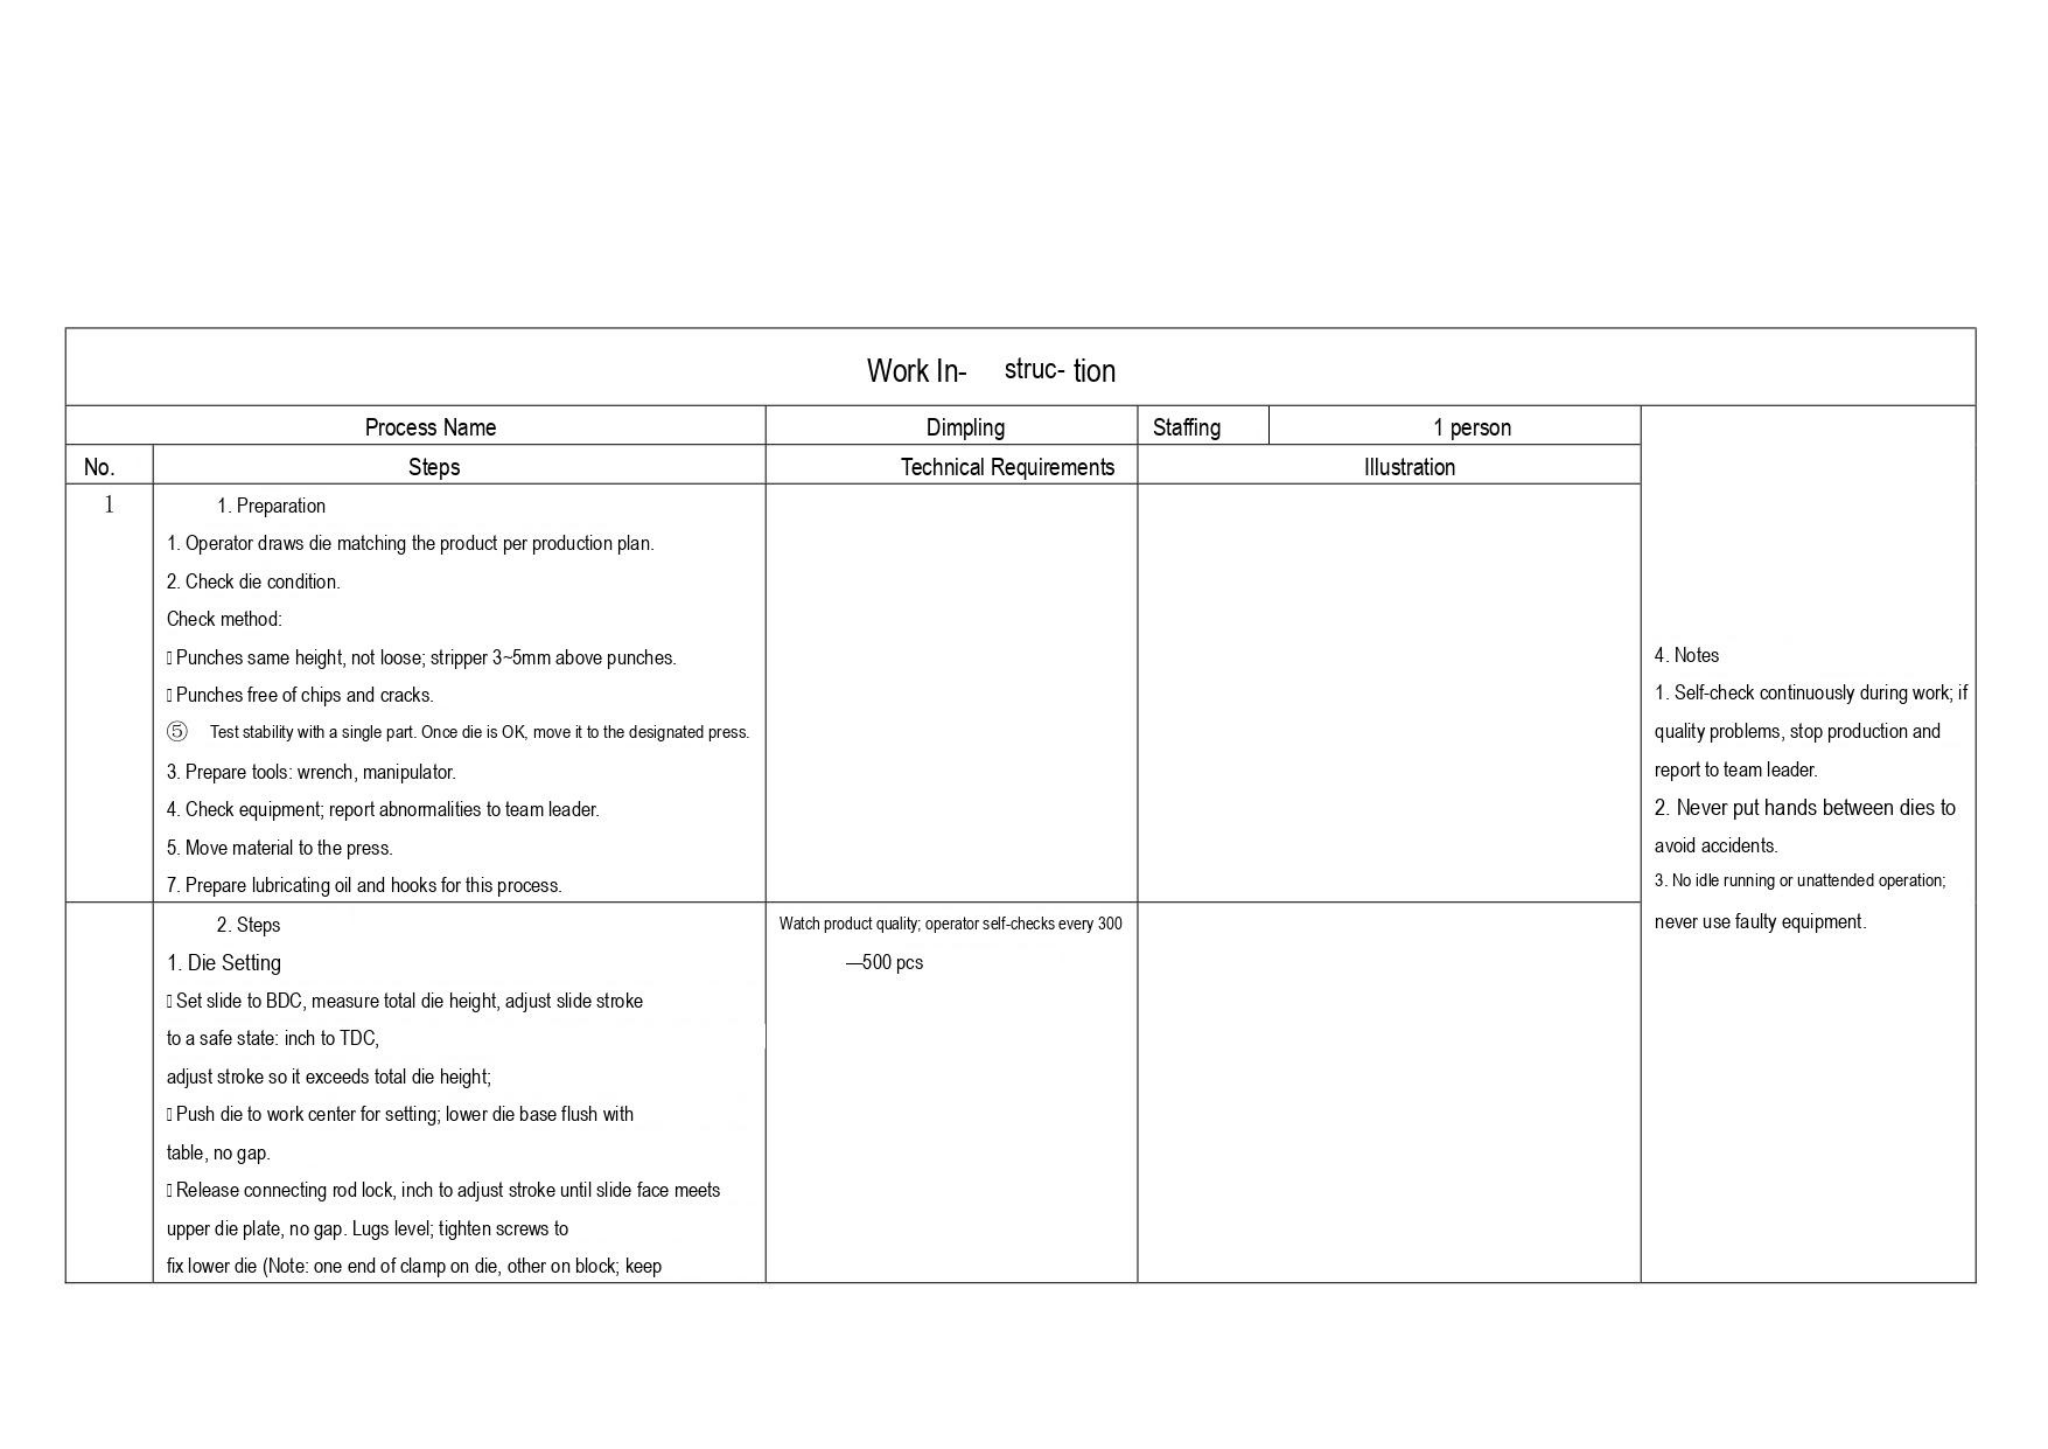# Work In- struc- tion

| Process Name | | Dimpling | Staffing | 1 person | |
|---|---|---|---|---|---|
| No. | Steps | Technical Requirements | Illustration | | |
| 1 | 1. Preparation<br>1. Operator draws die matching the product per production plan.<br>2. Check die condition.<br>Check method:<br>▯ Punches same height, not loose; stripper 3~5mm above punches.<br>▯ Punches free of chips and cracks.<br>⑤ Test stability with a single part. Once die is OK, move it to the designated press.<br>3. Prepare tools: wrench, manipulator.<br>4. Check equipment; report abnormalities to team leader.<br>5. Move material to the press.<br>7. Prepare lubricating oil and hooks for this process. | | | | 4. Notes<br>1. Self-check continuously during work; if quality problems, stop production and report to team leader.<br>2. Never put hands between dies to avoid accidents.<br>3. No idle running or unattended operation; never use faulty equipment. |
| | 2. Steps<br>1. Die Setting<br>▯ Set slide to BDC, measure total die height, adjust slide stroke to a safe state: inch to TDC,<br>adjust stroke so it exceeds total die height;<br>▯ Push die to work center for setting; lower die base flush with table, no gap.<br>▯ Release connecting rod lock, inch to adjust stroke until slide face meets upper die plate, no gap. Lugs level; tighten screws to fix lower die (Note: one end of clamp on die, other on block; keep | Watch product quality; operator self-checks every 300 —500 pcs | | | |
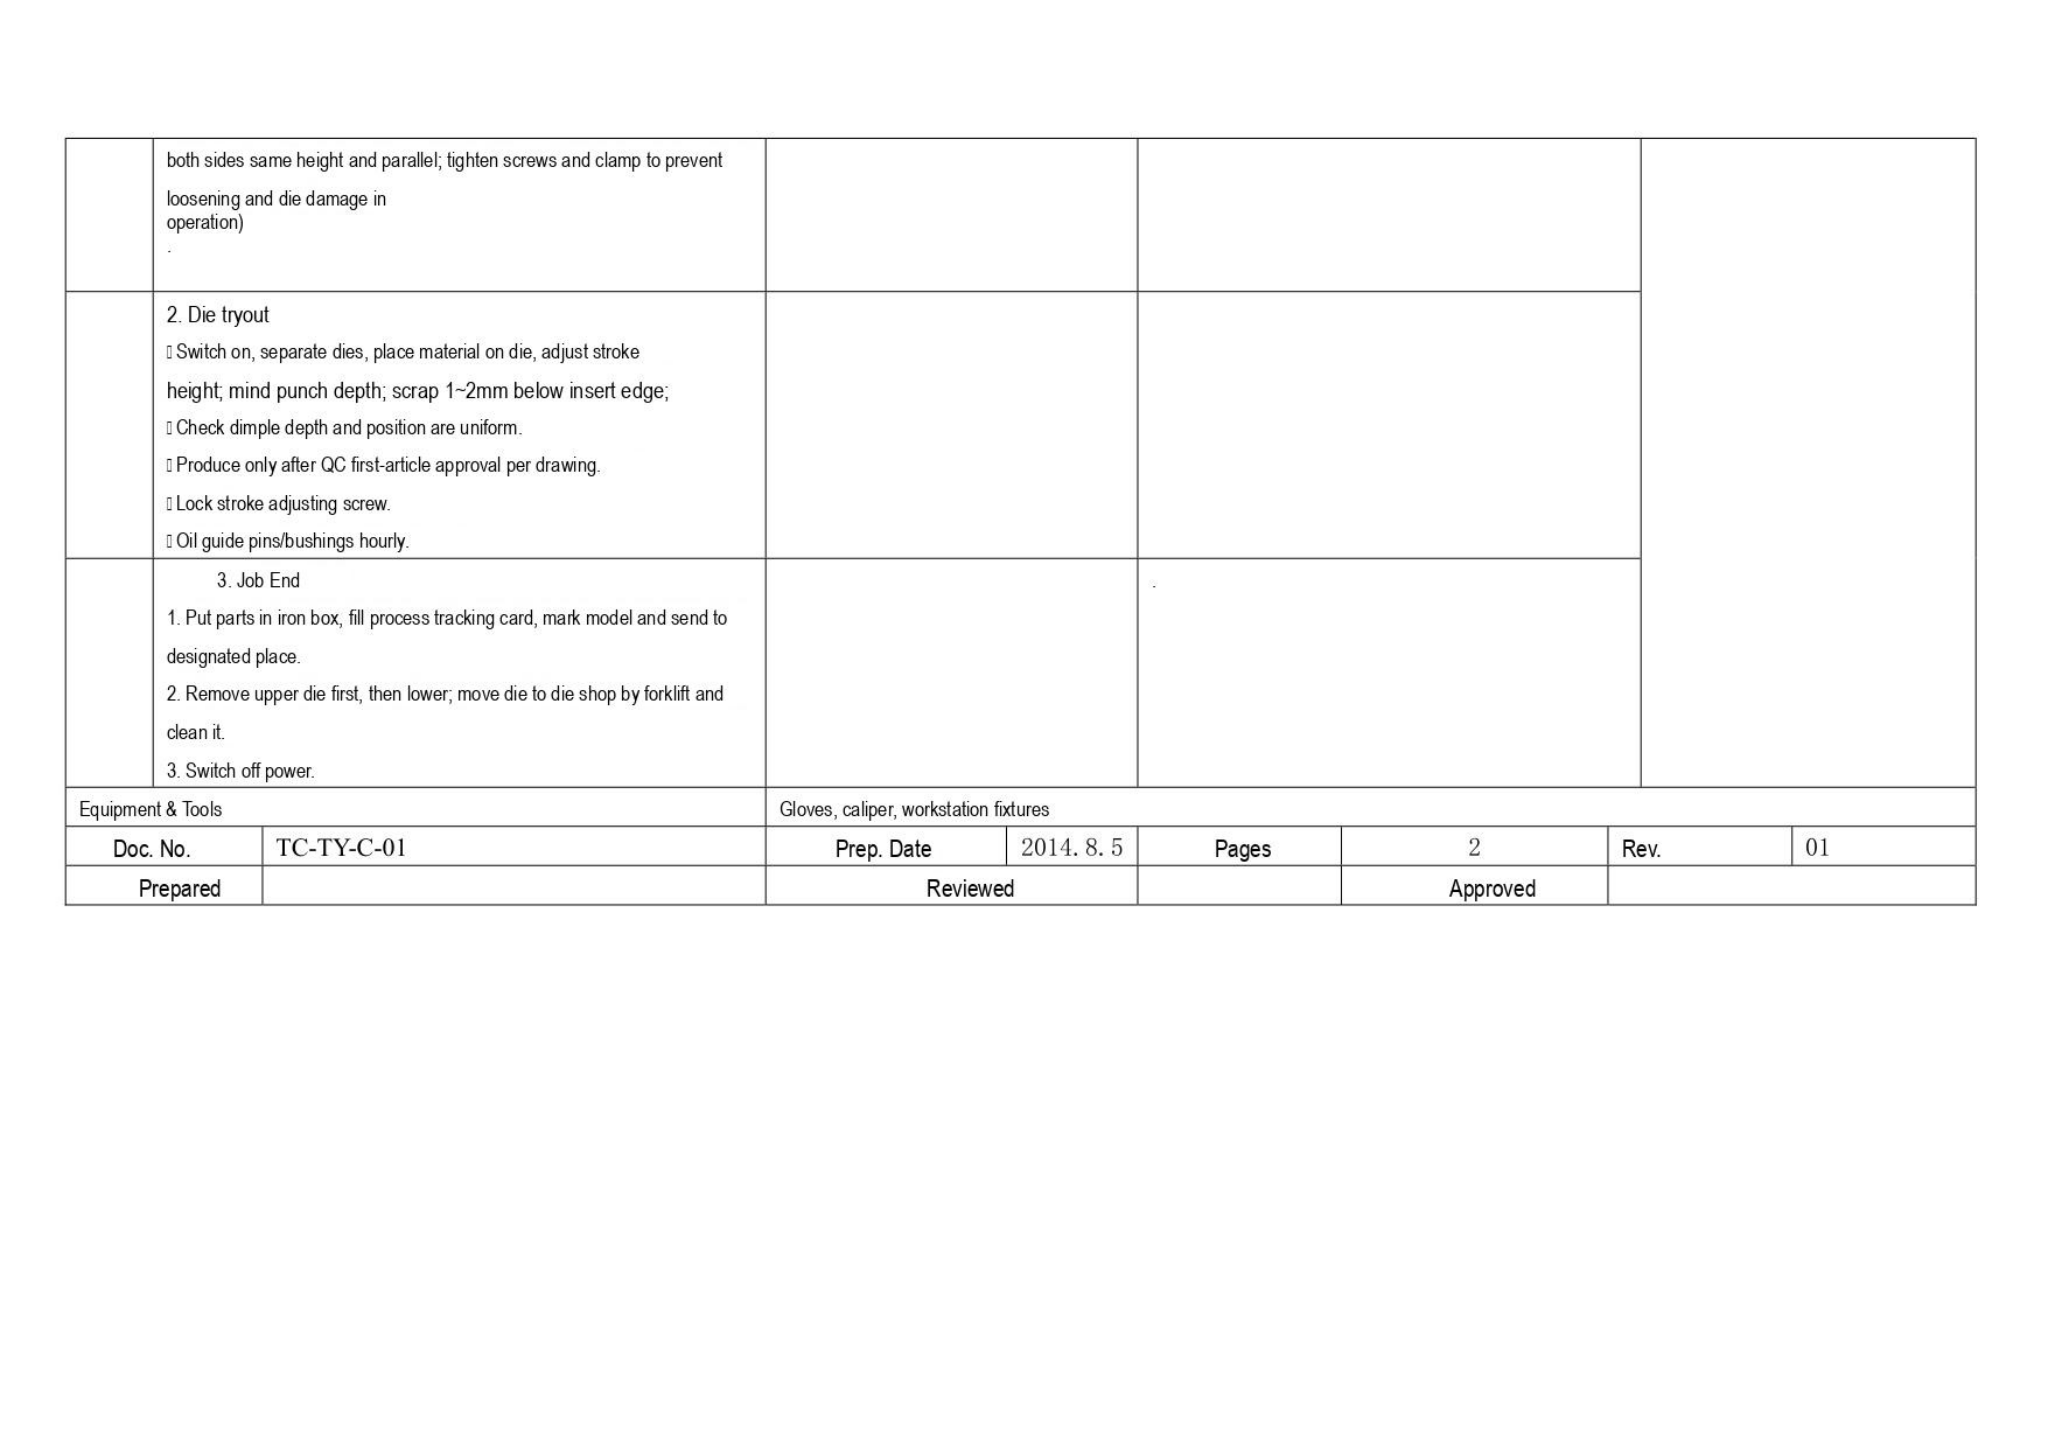| | | | | |
|---|---|---|---|---|
| | both sides same height and parallel; tighten screws and clamp to prevent loosening and die damage in operation) | | | |
| | 2. Die tryout<br>Switch on, separate dies, place material on die, adjust stroke height; mind punch depth; scrap 1~2mm below insert edge;<br>Check dimple depth and position are uniform.<br>Produce only after QC first-article approval per drawing.<br>Lock stroke adjusting screw.<br>Oil guide pins/bushings hourly. | | | |
| | 3. Job End<br>1. Put parts in iron box, fill process tracking card, mark model and send to designated place.<br>2. Remove upper die first, then lower; move die to die shop by forklift and clean it.<br>3. Switch off power. | | | |

| | | | | | | | |
|---|---|---|---|---|---|---|---|
| Equipment & Tools | | Gloves, caliper, workstation fixtures | | | | | |
| Doc. No. | TC-TY-C-01 | Prep. Date | 2014. 8. 5 | Pages | 2 | Rev. | 01 |
| Prepared | | Reviewed | | | Approved | | |